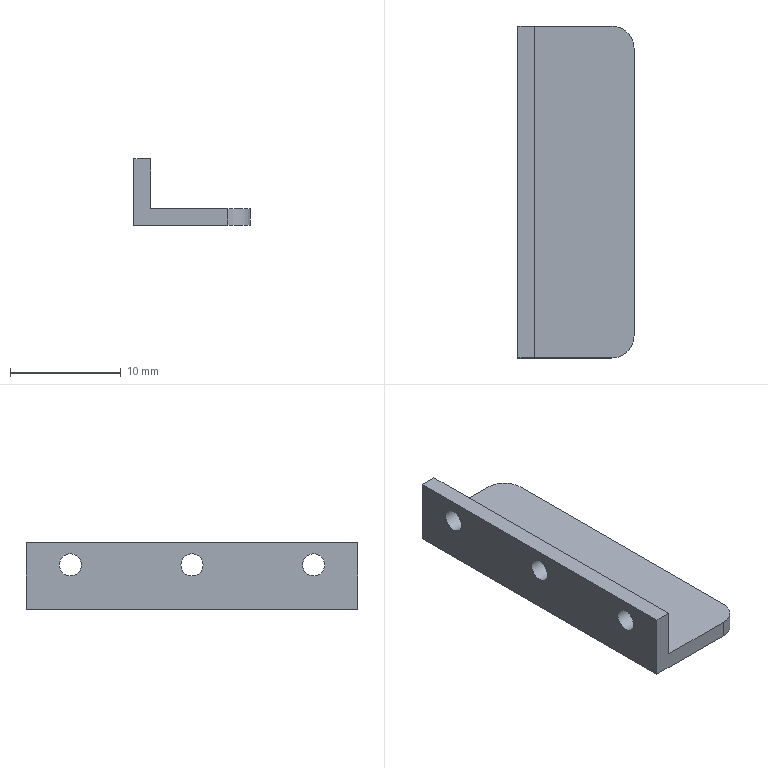Part | STEP file | 1-47.2 | 1 solid | 13 faces | box 10.5 x 30 x 6 mm | volume 658.288 mm3 | plane 8 | cylinder 5 | commonest cylinder face diameters 2 x3 4 x2
STEP:
#1=CARTESIAN_POINT('',(0.,0.,0.));
#2=DIRECTION('',(0.,0.,1.));
#3=DIRECTION('',(1.,0.,0.));
#4=AXIS2_PLACEMENT_3D('',#1,#2,#3);
#5=CARTESIAN_POINT('',(-1.5,-15.,-3.));
#6=VERTEX_POINT('',#5);
#7=CARTESIAN_POINT('',(-1.5,15.,-3.));
#8=VERTEX_POINT('',#7);
#9=CARTESIAN_POINT('',(-1.5,-15.,-3.));
#10=DIRECTION('',(0.,1.,0.));
#11=VECTOR('',#10,1.);
#12=LINE('',#9,#11);
#13=CARTESIAN_POINT('',(-1.5,0.,12.));
#14=DIRECTION('',(1.,0.,0.));
#15=DIRECTION('',(0.,1.,0.));
#16=AXIS2_PLACEMENT_3D('',#13,#14,#15);
#17=PLANE('',#16);
#18=CARTESIAN_POINT('',(-15.,-15.));
#19=DIRECTION('',(1.,0.));
#20=VECTOR('',#19,1.);
#21=LINE('',#18,#20);
#22=(GEOMETRIC_REPRESENTATION_CONTEXT(2)PARAMETRIC_REPRESENTATION_CONTEXT()REPRESENTATION_CONTEXT('',''));
#23=DEFINITIONAL_REPRESENTATION('',(#21),#22);
#24=PCURVE('',#17,#23);
#25=CARTESIAN_POINT('',(15.,0.,-3.));
#26=DIRECTION('',(0.,0.,1.));
#27=DIRECTION('',(0.,1.,0.));
#28=AXIS2_PLACEMENT_3D('',#25,#26,#27);
#29=PLANE('',#28);
#30=CARTESIAN_POINT('',(-15.,16.5));
#31=DIRECTION('',(1.,0.));
#32=VECTOR('',#31,1.);
#33=LINE('',#30,#32);
#34=(GEOMETRIC_REPRESENTATION_CONTEXT(2)PARAMETRIC_REPRESENTATION_CONTEXT()REPRESENTATION_CONTEXT('',''));
#35=DEFINITIONAL_REPRESENTATION('',(#33),#34);
#36=PCURVE('',#29,#35);
#37=SURFACE_CURVE('',#12,(#24,#36),.PCURVE_S1.);
#38=EDGE_CURVE('',#6,#8,#37,.T.);
#39=ORIENTED_EDGE('',*,*,#38,.T.);
#40=CARTESIAN_POINT('',(-1.5,15.,3.));
#41=VERTEX_POINT('',#40);
#42=CARTESIAN_POINT('',(-1.5,15.,-3.));
#43=DIRECTION('',(0.,0.,1.));
#44=VECTOR('',#43,1.);
#45=LINE('',#42,#44);
#46=CARTESIAN_POINT('',(15.,-15.));
#47=DIRECTION('',(0.,1.));
#48=VECTOR('',#47,1.);
#49=LINE('',#46,#48);
#50=(GEOMETRIC_REPRESENTATION_CONTEXT(2)PARAMETRIC_REPRESENTATION_CONTEXT()REPRESENTATION_CONTEXT('',''));
#51=DEFINITIONAL_REPRESENTATION('',(#49),#50);
#52=PCURVE('',#17,#51);
#53=CARTESIAN_POINT('',(3.75,15.,0.));
#54=DIRECTION('',(0.,-1.,0.));
#55=DIRECTION('',(0.,0.,1.));
#56=AXIS2_PLACEMENT_3D('',#53,#54,#55);
#57=PLANE('',#56);
#58=CARTESIAN_POINT('',(-3.,5.25));
#59=DIRECTION('',(1.,0.));
#60=VECTOR('',#59,1.);
#61=LINE('',#58,#60);
#62=(GEOMETRIC_REPRESENTATION_CONTEXT(2)PARAMETRIC_REPRESENTATION_CONTEXT()REPRESENTATION_CONTEXT('',''));
#63=DEFINITIONAL_REPRESENTATION('',(#61),#62);
#64=PCURVE('',#57,#63);
#65=SURFACE_CURVE('',#45,(#52,#64),.PCURVE_S1.);
#66=EDGE_CURVE('',#8,#41,#65,.T.);
#67=ORIENTED_EDGE('',*,*,#66,.T.);
#68=CARTESIAN_POINT('',(-1.5,-15.,3.));
#69=VERTEX_POINT('',#68);
#70=CARTESIAN_POINT('',(-1.5,15.,3.));
#71=DIRECTION('',(0.,-1.,0.));
#72=VECTOR('',#71,1.);
#73=LINE('',#70,#72);
#74=CARTESIAN_POINT('',(15.,-9.));
#75=DIRECTION('',(-1.,0.));
#76=VECTOR('',#75,1.);
#77=LINE('',#74,#76);
#78=(GEOMETRIC_REPRESENTATION_CONTEXT(2)PARAMETRIC_REPRESENTATION_CONTEXT()REPRESENTATION_CONTEXT('',''));
#79=DEFINITIONAL_REPRESENTATION('',(#77),#78);
#80=PCURVE('',#17,#79);
#81=CARTESIAN_POINT('',(-0.75,0.,3.));
#82=DIRECTION('',(0.,0.,-1.));
#83=DIRECTION('',(0.,-1.,0.));
#84=AXIS2_PLACEMENT_3D('',#81,#82,#83);
#85=PLANE('',#84);
#86=CARTESIAN_POINT('',(-15.,0.75));
#87=DIRECTION('',(1.,0.));
#88=VECTOR('',#87,1.);
#89=LINE('',#86,#88);
#90=(GEOMETRIC_REPRESENTATION_CONTEXT(2)PARAMETRIC_REPRESENTATION_CONTEXT()REPRESENTATION_CONTEXT('',''));
#91=DEFINITIONAL_REPRESENTATION('',(#89),#90);
#92=PCURVE('',#85,#91);
#93=SURFACE_CURVE('',#73,(#80,#92),.PCURVE_S1.);
#94=EDGE_CURVE('',#41,#69,#93,.T.);
#95=ORIENTED_EDGE('',*,*,#94,.T.);
#96=CARTESIAN_POINT('',(-1.5,-15.,3.));
#97=DIRECTION('',(0.,0.,-1.));
#98=VECTOR('',#97,1.);
#99=LINE('',#96,#98);
#100=CARTESIAN_POINT('',(-15.,-9.));
#101=DIRECTION('',(0.,-1.));
#102=VECTOR('',#101,1.);
#103=LINE('',#100,#102);
#104=(GEOMETRIC_REPRESENTATION_CONTEXT(2)PARAMETRIC_REPRESENTATION_CONTEXT()REPRESENTATION_CONTEXT('',''));
#105=DEFINITIONAL_REPRESENTATION('',(#103),#104);
#106=PCURVE('',#17,#105);
#107=CARTESIAN_POINT('',(3.75,-15.,0.));
#108=DIRECTION('',(0.,1.,0.));
#109=DIRECTION('',(0.,0.,-1.));
#110=AXIS2_PLACEMENT_3D('',#107,#108,#109);
#111=PLANE('',#110);
#112=CARTESIAN_POINT('',(-3.,5.25));
#113=DIRECTION('',(1.,0.));
#114=VECTOR('',#113,1.);
#115=LINE('',#112,#114);
#116=(GEOMETRIC_REPRESENTATION_CONTEXT(2)PARAMETRIC_REPRESENTATION_CONTEXT()REPRESENTATION_CONTEXT('',''));
#117=DEFINITIONAL_REPRESENTATION('',(#115),#116);
#118=PCURVE('',#111,#117);
#119=SURFACE_CURVE('',#99,(#106,#118),.PCURVE_S1.);
#120=EDGE_CURVE('',#69,#6,#119,.T.);
#121=ORIENTED_EDGE('',*,*,#120,.T.);
#122=EDGE_LOOP('',(#39,#67,#95,#121));
#123=FACE_BOUND('',#122,.F.);
#124=CARTESIAN_POINT('',(-1.5,1.,1.));
#125=VERTEX_POINT('',#124);
#126=CARTESIAN_POINT('',(-1.5,0.,1.));
#127=DIRECTION('',(-1.,0.,0.));
#128=DIRECTION('',(0.,1.,0.));
#129=AXIS2_PLACEMENT_3D('',#126,#127,#128);
#130=CIRCLE('',#129,1.);
#131=CARTESIAN_POINT('',(1.,-11.));
#132=CARTESIAN_POINT('',(1.,-12.732));
#133=CARTESIAN_POINT('',(-0.5,-11.866));
#134=CARTESIAN_POINT('',(-2.,-11.));
#135=CARTESIAN_POINT('',(-0.5,-10.134));
#136=CARTESIAN_POINT('',(1.,-9.268));
#137=CARTESIAN_POINT('',(1.,-11.));
#138=(BOUNDED_CURVE()B_SPLINE_CURVE(2,(#131,#132,#133,#134,#135,#136,#137),.UNSPECIFIED.,.T.,.F.)B_SPLINE_CURVE_WITH_KNOTS((1,2,2,2,2,1),(-2.094,0.,2.094,4.189,6.283,8.378),.UNSPECIFIED.)CURVE()GEOMETRIC_REPRESENTATION_ITEM()RATIONAL_B_SPLINE_CURVE((1.,0.5,1.,0.5,1.,0.5,1.))REPRESENTATION_ITEM(''));
#139=(GEOMETRIC_REPRESENTATION_CONTEXT(2)PARAMETRIC_REPRESENTATION_CONTEXT()REPRESENTATION_CONTEXT('',''));
#140=DEFINITIONAL_REPRESENTATION('',(#138),#139);
#141=PCURVE('',#17,#140);
#142=CARTESIAN_POINT('',(0.,0.,1.));
#143=DIRECTION('',(-1.,0.,0.));
#144=DIRECTION('',(0.,1.,0.));
#145=AXIS2_PLACEMENT_3D('',#142,#143,#144);
#146=CYLINDRICAL_SURFACE('',#145,1.);
#147=CARTESIAN_POINT('',(0.,1.5));
#148=DIRECTION('',(1.,0.));
#149=VECTOR('',#148,1.);
#150=LINE('',#147,#149);
#151=(GEOMETRIC_REPRESENTATION_CONTEXT(2)PARAMETRIC_REPRESENTATION_CONTEXT()REPRESENTATION_CONTEXT('',''));
#152=DEFINITIONAL_REPRESENTATION('',(#150),#151);
#153=PCURVE('',#146,#152);
#154=SURFACE_CURVE('',#130,(#141,#153),.PCURVE_S1.);
#155=EDGE_CURVE('',#125,#125,#154,.T.);
#156=ORIENTED_EDGE('',*,*,#155,.T.);
#157=EDGE_LOOP('',(#156));
#158=FACE_BOUND('',#157,.F.);
#159=CARTESIAN_POINT('',(-1.5,-10.,1.));
#160=VERTEX_POINT('',#159);
#161=CARTESIAN_POINT('',(-1.5,-11.,1.));
#162=DIRECTION('',(-1.,0.,0.));
#163=DIRECTION('',(0.,1.,0.));
#164=AXIS2_PLACEMENT_3D('',#161,#162,#163);
#165=CIRCLE('',#164,1.);
#166=CARTESIAN_POINT('',(-10.,-11.));
#167=CARTESIAN_POINT('',(-10.,-12.732));
#168=CARTESIAN_POINT('',(-11.5,-11.866));
#169=CARTESIAN_POINT('',(-13.,-11.));
#170=CARTESIAN_POINT('',(-11.5,-10.134));
#171=CARTESIAN_POINT('',(-10.,-9.268));
#172=CARTESIAN_POINT('',(-10.,-11.));
#173=(BOUNDED_CURVE()B_SPLINE_CURVE(2,(#166,#167,#168,#169,#170,#171,#172),.UNSPECIFIED.,.T.,.F.)B_SPLINE_CURVE_WITH_KNOTS((1,2,2,2,2,1),(-2.094,0.,2.094,4.189,6.283,8.378),.UNSPECIFIED.)CURVE()GEOMETRIC_REPRESENTATION_ITEM()RATIONAL_B_SPLINE_CURVE((1.,0.5,1.,0.5,1.,0.5,1.))REPRESENTATION_ITEM(''));
#174=(GEOMETRIC_REPRESENTATION_CONTEXT(2)PARAMETRIC_REPRESENTATION_CONTEXT()REPRESENTATION_CONTEXT('',''));
#175=DEFINITIONAL_REPRESENTATION('',(#173),#174);
#176=PCURVE('',#17,#175);
#177=CARTESIAN_POINT('',(0.,-11.,1.));
#178=DIRECTION('',(-1.,0.,0.));
#179=DIRECTION('',(0.,1.,0.));
#180=AXIS2_PLACEMENT_3D('',#177,#178,#179);
#181=CYLINDRICAL_SURFACE('',#180,1.);
#182=CARTESIAN_POINT('',(0.,1.5));
#183=DIRECTION('',(1.,0.));
#184=VECTOR('',#183,1.);
#185=LINE('',#182,#184);
#186=(GEOMETRIC_REPRESENTATION_CONTEXT(2)PARAMETRIC_REPRESENTATION_CONTEXT()REPRESENTATION_CONTEXT('',''));
#187=DEFINITIONAL_REPRESENTATION('',(#185),#186);
#188=PCURVE('',#181,#187);
#189=SURFACE_CURVE('',#165,(#176,#188),.PCURVE_S1.);
#190=EDGE_CURVE('',#160,#160,#189,.T.);
#191=ORIENTED_EDGE('',*,*,#190,.T.);
#192=EDGE_LOOP('',(#191));
#193=FACE_BOUND('',#192,.F.);
#194=CARTESIAN_POINT('',(-1.5,12.,1.));
#195=VERTEX_POINT('',#194);
#196=CARTESIAN_POINT('',(-1.5,11.,1.));
#197=DIRECTION('',(-1.,0.,0.));
#198=DIRECTION('',(0.,1.,0.));
#199=AXIS2_PLACEMENT_3D('',#196,#197,#198);
#200=CIRCLE('',#199,1.);
#201=CARTESIAN_POINT('',(12.,-11.));
#202=CARTESIAN_POINT('',(12.,-12.732));
#203=CARTESIAN_POINT('',(10.5,-11.866));
#204=CARTESIAN_POINT('',(9.,-11.));
#205=CARTESIAN_POINT('',(10.5,-10.134));
#206=CARTESIAN_POINT('',(12.,-9.268));
#207=CARTESIAN_POINT('',(12.,-11.));
#208=(BOUNDED_CURVE()B_SPLINE_CURVE(2,(#201,#202,#203,#204,#205,#206,#207),.UNSPECIFIED.,.T.,.F.)B_SPLINE_CURVE_WITH_KNOTS((1,2,2,2,2,1),(-2.094,0.,2.094,4.189,6.283,8.378),.UNSPECIFIED.)CURVE()GEOMETRIC_REPRESENTATION_ITEM()RATIONAL_B_SPLINE_CURVE((1.,0.5,1.,0.5,1.,0.5,1.))REPRESENTATION_ITEM(''));
#209=(GEOMETRIC_REPRESENTATION_CONTEXT(2)PARAMETRIC_REPRESENTATION_CONTEXT()REPRESENTATION_CONTEXT('',''));
#210=DEFINITIONAL_REPRESENTATION('',(#208),#209);
#211=PCURVE('',#17,#210);
#212=CARTESIAN_POINT('',(0.,11.,1.));
#213=DIRECTION('',(-1.,0.,0.));
#214=DIRECTION('',(0.,1.,0.));
#215=AXIS2_PLACEMENT_3D('',#212,#213,#214);
#216=CYLINDRICAL_SURFACE('',#215,1.);
#217=CARTESIAN_POINT('',(0.,1.5));
#218=DIRECTION('',(1.,0.));
#219=VECTOR('',#218,1.);
#220=LINE('',#217,#219);
#221=(GEOMETRIC_REPRESENTATION_CONTEXT(2)PARAMETRIC_REPRESENTATION_CONTEXT()REPRESENTATION_CONTEXT('',''));
#222=DEFINITIONAL_REPRESENTATION('',(#220),#221);
#223=PCURVE('',#216,#222);
#224=SURFACE_CURVE('',#200,(#211,#223),.PCURVE_S1.);
#225=EDGE_CURVE('',#195,#195,#224,.T.);
#226=ORIENTED_EDGE('',*,*,#225,.T.);
#227=EDGE_LOOP('',(#226));
#228=FACE_BOUND('',#227,.F.);
#229=ADVANCED_FACE('',(#123,#158,#193,#228),#17,.F.);
#230=CARTESIAN_POINT('',(0.,15.,3.));
#231=VERTEX_POINT('',#230);
#232=CARTESIAN_POINT('',(0.,-15.,3.));
#233=VERTEX_POINT('',#232);
#234=CARTESIAN_POINT('',(0.,15.,3.));
#235=DIRECTION('',(0.,-1.,0.));
#236=VECTOR('',#235,1.);
#237=LINE('',#234,#236);
#238=CARTESIAN_POINT('',(-15.,-0.75));
#239=DIRECTION('',(1.,0.));
#240=VECTOR('',#239,1.);
#241=LINE('',#238,#240);
#242=(GEOMETRIC_REPRESENTATION_CONTEXT(2)PARAMETRIC_REPRESENTATION_CONTEXT()REPRESENTATION_CONTEXT('',''));
#243=DEFINITIONAL_REPRESENTATION('',(#241),#242);
#244=PCURVE('',#85,#243);
#245=CARTESIAN_POINT('',(0.,0.,12.));
#246=DIRECTION('',(1.,0.,0.));
#247=DIRECTION('',(0.,1.,0.));
#248=AXIS2_PLACEMENT_3D('',#245,#246,#247);
#249=PLANE('',#248);
#250=CARTESIAN_POINT('',(15.,-9.));
#251=DIRECTION('',(-1.,0.));
#252=VECTOR('',#251,1.);
#253=LINE('',#250,#252);
#254=(GEOMETRIC_REPRESENTATION_CONTEXT(2)PARAMETRIC_REPRESENTATION_CONTEXT()REPRESENTATION_CONTEXT('',''));
#255=DEFINITIONAL_REPRESENTATION('',(#253),#254);
#256=PCURVE('',#249,#255);
#257=SURFACE_CURVE('',#237,(#244,#256),.PCURVE_S1.);
#258=EDGE_CURVE('',#231,#233,#257,.T.);
#259=ORIENTED_EDGE('',*,*,#258,.T.);
#260=CARTESIAN_POINT('',(0.,-15.,3.));
#261=DIRECTION('',(-1.,0.,0.));
#262=VECTOR('',#261,1.);
#263=LINE('',#260,#262);
#264=CARTESIAN_POINT('',(15.,-0.75));
#265=DIRECTION('',(0.,1.));
#266=VECTOR('',#265,1.);
#267=LINE('',#264,#266);
#268=(GEOMETRIC_REPRESENTATION_CONTEXT(2)PARAMETRIC_REPRESENTATION_CONTEXT()REPRESENTATION_CONTEXT('',''));
#269=DEFINITIONAL_REPRESENTATION('',(#267),#268);
#270=PCURVE('',#85,#269);
#271=CARTESIAN_POINT('',(-3.,3.75));
#272=DIRECTION('',(0.,1.));
#273=VECTOR('',#272,1.);
#274=LINE('',#271,#273);
#275=(GEOMETRIC_REPRESENTATION_CONTEXT(2)PARAMETRIC_REPRESENTATION_CONTEXT()REPRESENTATION_CONTEXT('',''));
#276=DEFINITIONAL_REPRESENTATION('',(#274),#275);
#277=PCURVE('',#111,#276);
#278=SURFACE_CURVE('',#263,(#270,#277),.PCURVE_S1.);
#279=EDGE_CURVE('',#233,#69,#278,.T.);
#280=ORIENTED_EDGE('',*,*,#279,.T.);
#281=ORIENTED_EDGE('',*,*,#94,.F.);
#282=CARTESIAN_POINT('',(0.,15.,3.));
#283=DIRECTION('',(-1.,0.,0.));
#284=VECTOR('',#283,1.);
#285=LINE('',#282,#284);
#286=CARTESIAN_POINT('',(-15.,-0.75));
#287=DIRECTION('',(0.,1.));
#288=VECTOR('',#287,1.);
#289=LINE('',#286,#288);
#290=(GEOMETRIC_REPRESENTATION_CONTEXT(2)PARAMETRIC_REPRESENTATION_CONTEXT()REPRESENTATION_CONTEXT('',''));
#291=DEFINITIONAL_REPRESENTATION('',(#289),#290);
#292=PCURVE('',#85,#291);
#293=CARTESIAN_POINT('',(3.,3.75));
#294=DIRECTION('',(0.,1.));
#295=VECTOR('',#294,1.);
#296=LINE('',#293,#295);
#297=(GEOMETRIC_REPRESENTATION_CONTEXT(2)PARAMETRIC_REPRESENTATION_CONTEXT()REPRESENTATION_CONTEXT('',''));
#298=DEFINITIONAL_REPRESENTATION('',(#296),#297);
#299=PCURVE('',#57,#298);
#300=SURFACE_CURVE('',#285,(#292,#299),.PCURVE_S1.);
#301=EDGE_CURVE('',#231,#41,#300,.T.);
#302=ORIENTED_EDGE('',*,*,#301,.F.);
#303=EDGE_LOOP('',(#259,#280,#281,#302));
#304=FACE_BOUND('',#303,.F.);
#305=ADVANCED_FACE('',(#304),#85,.F.);
#306=CARTESIAN_POINT('',(0.,1.,1.));
#307=VERTEX_POINT('',#306);
#308=CARTESIAN_POINT('',(0.,0.,1.));
#309=DIRECTION('',(-1.,0.,0.));
#310=DIRECTION('',(0.,1.,0.));
#311=AXIS2_PLACEMENT_3D('',#308,#309,#310);
#312=CIRCLE('',#311,1.);
#313=CARTESIAN_POINT('',(0.,0.));
#314=DIRECTION('',(1.,0.));
#315=VECTOR('',#314,1.);
#316=LINE('',#313,#315);
#317=(GEOMETRIC_REPRESENTATION_CONTEXT(2)PARAMETRIC_REPRESENTATION_CONTEXT()REPRESENTATION_CONTEXT('',''));
#318=DEFINITIONAL_REPRESENTATION('',(#316),#317);
#319=PCURVE('',#146,#318);
#320=CARTESIAN_POINT('',(1.,-11.));
#321=CARTESIAN_POINT('',(1.,-12.732));
#322=CARTESIAN_POINT('',(-0.5,-11.866));
#323=CARTESIAN_POINT('',(-2.,-11.));
#324=CARTESIAN_POINT('',(-0.5,-10.134));
#325=CARTESIAN_POINT('',(1.,-9.268));
#326=CARTESIAN_POINT('',(1.,-11.));
#327=(BOUNDED_CURVE()B_SPLINE_CURVE(2,(#320,#321,#322,#323,#324,#325,#326),.UNSPECIFIED.,.T.,.F.)B_SPLINE_CURVE_WITH_KNOTS((1,2,2,2,2,1),(-2.094,0.,2.094,4.189,6.283,8.378),.UNSPECIFIED.)CURVE()GEOMETRIC_REPRESENTATION_ITEM()RATIONAL_B_SPLINE_CURVE((1.,0.5,1.,0.5,1.,0.5,1.))REPRESENTATION_ITEM(''));
#328=(GEOMETRIC_REPRESENTATION_CONTEXT(2)PARAMETRIC_REPRESENTATION_CONTEXT()REPRESENTATION_CONTEXT('',''));
#329=DEFINITIONAL_REPRESENTATION('',(#327),#328);
#330=PCURVE('',#249,#329);
#331=SURFACE_CURVE('',#312,(#319,#330),.PCURVE_S1.);
#332=EDGE_CURVE('',#307,#307,#331,.T.);
#333=ORIENTED_EDGE('',*,*,#332,.T.);
#334=CARTESIAN_POINT('',(0.,1.,1.));
#335=DIRECTION('',(-1.,0.,0.));
#336=VECTOR('',#335,1.);
#337=LINE('',#334,#336);
#338=CARTESIAN_POINT('',(6.283,0.));
#339=DIRECTION('',(0.,1.));
#340=VECTOR('',#339,1.);
#341=LINE('',#338,#340);
#342=(GEOMETRIC_REPRESENTATION_CONTEXT(2)PARAMETRIC_REPRESENTATION_CONTEXT()REPRESENTATION_CONTEXT('',''));
#343=DEFINITIONAL_REPRESENTATION('',(#341),#342);
#344=PCURVE('',#146,#343);
#345=CARTESIAN_POINT('',(0.,0.));
#346=DIRECTION('',(0.,1.));
#347=VECTOR('',#346,1.);
#348=LINE('',#345,#347);
#349=(GEOMETRIC_REPRESENTATION_CONTEXT(2)PARAMETRIC_REPRESENTATION_CONTEXT()REPRESENTATION_CONTEXT('',''));
#350=DEFINITIONAL_REPRESENTATION('',(#348),#349);
#351=PCURVE('',#146,#350);
#352=SEAM_CURVE('',#337,(#344,#351),.PCURVE_S1.);
#353=EDGE_CURVE('',#307,#125,#352,.T.);
#354=ORIENTED_EDGE('',*,*,#353,.T.);
#355=ORIENTED_EDGE('',*,*,#155,.F.);
#356=ORIENTED_EDGE('',*,*,#353,.F.);
#357=EDGE_LOOP('',(#333,#354,#355,#356));
#358=FACE_BOUND('',#357,.F.);
#359=ADVANCED_FACE('',(#358),#146,.F.);
#360=CARTESIAN_POINT('',(0.,-10.,1.));
#361=VERTEX_POINT('',#360);
#362=CARTESIAN_POINT('',(0.,-11.,1.));
#363=DIRECTION('',(-1.,0.,0.));
#364=DIRECTION('',(0.,1.,0.));
#365=AXIS2_PLACEMENT_3D('',#362,#363,#364);
#366=CIRCLE('',#365,1.);
#367=CARTESIAN_POINT('',(0.,0.));
#368=DIRECTION('',(1.,0.));
#369=VECTOR('',#368,1.);
#370=LINE('',#367,#369);
#371=(GEOMETRIC_REPRESENTATION_CONTEXT(2)PARAMETRIC_REPRESENTATION_CONTEXT()REPRESENTATION_CONTEXT('',''));
#372=DEFINITIONAL_REPRESENTATION('',(#370),#371);
#373=PCURVE('',#181,#372);
#374=CARTESIAN_POINT('',(-10.,-11.));
#375=CARTESIAN_POINT('',(-10.,-12.732));
#376=CARTESIAN_POINT('',(-11.5,-11.866));
#377=CARTESIAN_POINT('',(-13.,-11.));
#378=CARTESIAN_POINT('',(-11.5,-10.134));
#379=CARTESIAN_POINT('',(-10.,-9.268));
#380=CARTESIAN_POINT('',(-10.,-11.));
#381=(BOUNDED_CURVE()B_SPLINE_CURVE(2,(#374,#375,#376,#377,#378,#379,#380),.UNSPECIFIED.,.T.,.F.)B_SPLINE_CURVE_WITH_KNOTS((1,2,2,2,2,1),(-2.094,0.,2.094,4.189,6.283,8.378),.UNSPECIFIED.)CURVE()GEOMETRIC_REPRESENTATION_ITEM()RATIONAL_B_SPLINE_CURVE((1.,0.5,1.,0.5,1.,0.5,1.))REPRESENTATION_ITEM(''));
#382=(GEOMETRIC_REPRESENTATION_CONTEXT(2)PARAMETRIC_REPRESENTATION_CONTEXT()REPRESENTATION_CONTEXT('',''));
#383=DEFINITIONAL_REPRESENTATION('',(#381),#382);
#384=PCURVE('',#249,#383);
#385=SURFACE_CURVE('',#366,(#373,#384),.PCURVE_S1.);
#386=EDGE_CURVE('',#361,#361,#385,.T.);
#387=ORIENTED_EDGE('',*,*,#386,.T.);
#388=CARTESIAN_POINT('',(0.,-10.,1.));
#389=DIRECTION('',(-1.,0.,0.));
#390=VECTOR('',#389,1.);
#391=LINE('',#388,#390);
#392=CARTESIAN_POINT('',(6.283,0.));
#393=DIRECTION('',(0.,1.));
#394=VECTOR('',#393,1.);
#395=LINE('',#392,#394);
#396=(GEOMETRIC_REPRESENTATION_CONTEXT(2)PARAMETRIC_REPRESENTATION_CONTEXT()REPRESENTATION_CONTEXT('',''));
#397=DEFINITIONAL_REPRESENTATION('',(#395),#396);
#398=PCURVE('',#181,#397);
#399=CARTESIAN_POINT('',(0.,0.));
#400=DIRECTION('',(0.,1.));
#401=VECTOR('',#400,1.);
#402=LINE('',#399,#401);
#403=(GEOMETRIC_REPRESENTATION_CONTEXT(2)PARAMETRIC_REPRESENTATION_CONTEXT()REPRESENTATION_CONTEXT('',''));
#404=DEFINITIONAL_REPRESENTATION('',(#402),#403);
#405=PCURVE('',#181,#404);
#406=SEAM_CURVE('',#391,(#398,#405),.PCURVE_S1.);
#407=EDGE_CURVE('',#361,#160,#406,.T.);
#408=ORIENTED_EDGE('',*,*,#407,.T.);
#409=ORIENTED_EDGE('',*,*,#190,.F.);
#410=ORIENTED_EDGE('',*,*,#407,.F.);
#411=EDGE_LOOP('',(#387,#408,#409,#410));
#412=FACE_BOUND('',#411,.F.);
#413=ADVANCED_FACE('',(#412),#181,.F.);
#414=CARTESIAN_POINT('',(0.,12.,1.));
#415=VERTEX_POINT('',#414);
#416=CARTESIAN_POINT('',(0.,11.,1.));
#417=DIRECTION('',(-1.,0.,0.));
#418=DIRECTION('',(0.,1.,0.));
#419=AXIS2_PLACEMENT_3D('',#416,#417,#418);
#420=CIRCLE('',#419,1.);
#421=CARTESIAN_POINT('',(0.,0.));
#422=DIRECTION('',(1.,0.));
#423=VECTOR('',#422,1.);
#424=LINE('',#421,#423);
#425=(GEOMETRIC_REPRESENTATION_CONTEXT(2)PARAMETRIC_REPRESENTATION_CONTEXT()REPRESENTATION_CONTEXT('',''));
#426=DEFINITIONAL_REPRESENTATION('',(#424),#425);
#427=PCURVE('',#216,#426);
#428=CARTESIAN_POINT('',(12.,-11.));
#429=CARTESIAN_POINT('',(12.,-12.732));
#430=CARTESIAN_POINT('',(10.5,-11.866));
#431=CARTESIAN_POINT('',(9.,-11.));
#432=CARTESIAN_POINT('',(10.5,-10.134));
#433=CARTESIAN_POINT('',(12.,-9.268));
#434=CARTESIAN_POINT('',(12.,-11.));
#435=(BOUNDED_CURVE()B_SPLINE_CURVE(2,(#428,#429,#430,#431,#432,#433,#434),.UNSPECIFIED.,.T.,.F.)B_SPLINE_CURVE_WITH_KNOTS((1,2,2,2,2,1),(-2.094,0.,2.094,4.189,6.283,8.378),.UNSPECIFIED.)CURVE()GEOMETRIC_REPRESENTATION_ITEM()RATIONAL_B_SPLINE_CURVE((1.,0.5,1.,0.5,1.,0.5,1.))REPRESENTATION_ITEM(''));
#436=(GEOMETRIC_REPRESENTATION_CONTEXT(2)PARAMETRIC_REPRESENTATION_CONTEXT()REPRESENTATION_CONTEXT('',''));
#437=DEFINITIONAL_REPRESENTATION('',(#435),#436);
#438=PCURVE('',#249,#437);
#439=SURFACE_CURVE('',#420,(#427,#438),.PCURVE_S1.);
#440=EDGE_CURVE('',#415,#415,#439,.T.);
#441=ORIENTED_EDGE('',*,*,#440,.T.);
#442=CARTESIAN_POINT('',(0.,12.,1.));
#443=DIRECTION('',(-1.,0.,0.));
#444=VECTOR('',#443,1.);
#445=LINE('',#442,#444);
#446=CARTESIAN_POINT('',(6.283,0.));
#447=DIRECTION('',(0.,1.));
#448=VECTOR('',#447,1.);
#449=LINE('',#446,#448);
#450=(GEOMETRIC_REPRESENTATION_CONTEXT(2)PARAMETRIC_REPRESENTATION_CONTEXT()REPRESENTATION_CONTEXT('',''));
#451=DEFINITIONAL_REPRESENTATION('',(#449),#450);
#452=PCURVE('',#216,#451);
#453=CARTESIAN_POINT('',(0.,0.));
#454=DIRECTION('',(0.,1.));
#455=VECTOR('',#454,1.);
#456=LINE('',#453,#455);
#457=(GEOMETRIC_REPRESENTATION_CONTEXT(2)PARAMETRIC_REPRESENTATION_CONTEXT()REPRESENTATION_CONTEXT('',''));
#458=DEFINITIONAL_REPRESENTATION('',(#456),#457);
#459=PCURVE('',#216,#458);
#460=SEAM_CURVE('',#445,(#452,#459),.PCURVE_S1.);
#461=EDGE_CURVE('',#415,#195,#460,.T.);
#462=ORIENTED_EDGE('',*,*,#461,.T.);
#463=ORIENTED_EDGE('',*,*,#225,.F.);
#464=ORIENTED_EDGE('',*,*,#461,.F.);
#465=EDGE_LOOP('',(#441,#462,#463,#464));
#466=FACE_BOUND('',#465,.F.);
#467=ADVANCED_FACE('',(#466),#216,.F.);
#468=ORIENTED_EDGE('',*,*,#258,.T.);
#469=CARTESIAN_POINT('',(0.,-15.,-1.5));
#470=VERTEX_POINT('',#469);
#471=CARTESIAN_POINT('',(0.,-15.,3.));
#472=DIRECTION('',(0.,0.,-1.));
#473=VECTOR('',#472,1.);
#474=LINE('',#471,#473);
#475=CARTESIAN_POINT('',(-15.,-9.));
#476=DIRECTION('',(0.,-1.));
#477=VECTOR('',#476,1.);
#478=LINE('',#475,#477);
#479=(GEOMETRIC_REPRESENTATION_CONTEXT(2)PARAMETRIC_REPRESENTATION_CONTEXT()REPRESENTATION_CONTEXT('',''));
#480=DEFINITIONAL_REPRESENTATION('',(#478),#479);
#481=PCURVE('',#249,#480);
#482=CARTESIAN_POINT('',(-3.,3.75));
#483=DIRECTION('',(1.,0.));
#484=VECTOR('',#483,1.);
#485=LINE('',#482,#484);
#486=(GEOMETRIC_REPRESENTATION_CONTEXT(2)PARAMETRIC_REPRESENTATION_CONTEXT()REPRESENTATION_CONTEXT('',''));
#487=DEFINITIONAL_REPRESENTATION('',(#485),#486);
#488=PCURVE('',#111,#487);
#489=SURFACE_CURVE('',#474,(#481,#488),.PCURVE_S1.);
#490=EDGE_CURVE('',#233,#470,#489,.T.);
#491=ORIENTED_EDGE('',*,*,#490,.T.);
#492=CARTESIAN_POINT('',(0.,15.,-1.5));
#493=VERTEX_POINT('',#492);
#494=CARTESIAN_POINT('',(0.,-15.,-1.5));
#495=DIRECTION('',(0.,1.,0.));
#496=VECTOR('',#495,1.);
#497=LINE('',#494,#496);
#498=CARTESIAN_POINT('',(-15.,-13.5));
#499=DIRECTION('',(1.,0.));
#500=VECTOR('',#499,1.);
#501=LINE('',#498,#500);
#502=(GEOMETRIC_REPRESENTATION_CONTEXT(2)PARAMETRIC_REPRESENTATION_CONTEXT()REPRESENTATION_CONTEXT('',''));
#503=DEFINITIONAL_REPRESENTATION('',(#501),#502);
#504=PCURVE('',#249,#503);
#505=CARTESIAN_POINT('',(15.,1.682,-1.5));
#506=DIRECTION('',(0.,0.,-1.));
#507=DIRECTION('',(0.,1.,0.));
#508=AXIS2_PLACEMENT_3D('',#505,#506,#507);
#509=PLANE('',#508);
#510=CARTESIAN_POINT('',(-16.682,-15.));
#511=DIRECTION('',(1.,0.));
#512=VECTOR('',#511,1.);
#513=LINE('',#510,#512);
#514=(GEOMETRIC_REPRESENTATION_CONTEXT(2)PARAMETRIC_REPRESENTATION_CONTEXT()REPRESENTATION_CONTEXT('',''));
#515=DEFINITIONAL_REPRESENTATION('',(#513),#514);
#516=PCURVE('',#509,#515);
#517=SURFACE_CURVE('',#497,(#504,#516),.PCURVE_S1.);
#518=EDGE_CURVE('',#470,#493,#517,.T.);
#519=ORIENTED_EDGE('',*,*,#518,.T.);
#520=CARTESIAN_POINT('',(0.,15.,-1.5));
#521=DIRECTION('',(0.,0.,1.));
#522=VECTOR('',#521,1.);
#523=LINE('',#520,#522);
#524=CARTESIAN_POINT('',(15.,-13.5));
#525=DIRECTION('',(0.,1.));
#526=VECTOR('',#525,1.);
#527=LINE('',#524,#526);
#528=(GEOMETRIC_REPRESENTATION_CONTEXT(2)PARAMETRIC_REPRESENTATION_CONTEXT()REPRESENTATION_CONTEXT('',''));
#529=DEFINITIONAL_REPRESENTATION('',(#527),#528);
#530=PCURVE('',#249,#529);
#531=CARTESIAN_POINT('',(-1.5,3.75));
#532=DIRECTION('',(1.,0.));
#533=VECTOR('',#532,1.);
#534=LINE('',#531,#533);
#535=(GEOMETRIC_REPRESENTATION_CONTEXT(2)PARAMETRIC_REPRESENTATION_CONTEXT()REPRESENTATION_CONTEXT('',''));
#536=DEFINITIONAL_REPRESENTATION('',(#534),#535);
#537=PCURVE('',#57,#536);
#538=SURFACE_CURVE('',#523,(#530,#537),.PCURVE_S1.);
#539=EDGE_CURVE('',#493,#231,#538,.T.);
#540=ORIENTED_EDGE('',*,*,#539,.T.);
#541=EDGE_LOOP('',(#468,#491,#519,#540));
#542=FACE_BOUND('',#541,.T.);
#543=ORIENTED_EDGE('',*,*,#332,.T.);
#544=EDGE_LOOP('',(#543));
#545=FACE_BOUND('',#544,.T.);
#546=ORIENTED_EDGE('',*,*,#386,.T.);
#547=EDGE_LOOP('',(#546));
#548=FACE_BOUND('',#547,.T.);
#549=ORIENTED_EDGE('',*,*,#440,.T.);
#550=EDGE_LOOP('',(#549));
#551=FACE_BOUND('',#550,.T.);
#552=ADVANCED_FACE('',(#542,#545,#548,#551),#249,.T.);
#553=ORIENTED_EDGE('',*,*,#38,.F.);
#554=CARTESIAN_POINT('',(7.,-15.,-3.));
#555=VERTEX_POINT('',#554);
#556=CARTESIAN_POINT('',(-1.5,-15.,-3.));
#557=DIRECTION('',(1.,0.,0.));
#558=VECTOR('',#557,1.);
#559=LINE('',#556,#558);
#560=CARTESIAN_POINT('',(-15.,16.5));
#561=DIRECTION('',(0.,-1.));
#562=VECTOR('',#561,1.);
#563=LINE('',#560,#562);
#564=(GEOMETRIC_REPRESENTATION_CONTEXT(2)PARAMETRIC_REPRESENTATION_CONTEXT()REPRESENTATION_CONTEXT('',''));
#565=DEFINITIONAL_REPRESENTATION('',(#563),#564);
#566=PCURVE('',#29,#565);
#567=CARTESIAN_POINT('',(3.,5.25));
#568=DIRECTION('',(0.,-1.));
#569=VECTOR('',#568,1.);
#570=LINE('',#567,#569);
#571=(GEOMETRIC_REPRESENTATION_CONTEXT(2)PARAMETRIC_REPRESENTATION_CONTEXT()REPRESENTATION_CONTEXT('',''));
#572=DEFINITIONAL_REPRESENTATION('',(#570),#571);
#573=PCURVE('',#111,#572);
#574=SURFACE_CURVE('',#559,(#566,#573),.PCURVE_S1.);
#575=EDGE_CURVE('',#6,#555,#574,.T.);
#576=ORIENTED_EDGE('',*,*,#575,.T.);
#577=CARTESIAN_POINT('',(9.,-13.,-3.));
#578=VERTEX_POINT('',#577);
#579=CARTESIAN_POINT('',(7.,-13.,-3.));
#580=DIRECTION('',(0.,0.,-1.));
#581=DIRECTION('',(1.,0.,0.));
#582=AXIS2_PLACEMENT_3D('',#579,#580,#581);
#583=CIRCLE('',#582,2.);
#584=CARTESIAN_POINT('',(-13.,6.));
#585=CARTESIAN_POINT('',(-16.464,6.));
#586=CARTESIAN_POINT('',(-14.732,9.));
#587=CARTESIAN_POINT('',(-13.,12.));
#588=CARTESIAN_POINT('',(-11.268,9.));
#589=CARTESIAN_POINT('',(-9.536,6.));
#590=CARTESIAN_POINT('',(-13.,6.));
#591=(BOUNDED_CURVE()B_SPLINE_CURVE(2,(#584,#585,#586,#587,#588,#589,#590),.UNSPECIFIED.,.T.,.F.)B_SPLINE_CURVE_WITH_KNOTS((1,2,2,2,2,1),(-2.094,0.,2.094,4.189,6.283,8.378),.UNSPECIFIED.)CURVE()GEOMETRIC_REPRESENTATION_ITEM()RATIONAL_B_SPLINE_CURVE((1.,0.5,1.,0.5,1.,0.5,1.))REPRESENTATION_ITEM(''));
#592=(GEOMETRIC_REPRESENTATION_CONTEXT(2)PARAMETRIC_REPRESENTATION_CONTEXT()REPRESENTATION_CONTEXT('',''));
#593=DEFINITIONAL_REPRESENTATION('',(#591),#592);
#594=PCURVE('',#29,#593);
#595=CARTESIAN_POINT('',(7.,-13.,-3.));
#596=DIRECTION('',(0.,0.,1.));
#597=DIRECTION('',(1.,0.,0.));
#598=AXIS2_PLACEMENT_3D('',#595,#596,#597);
#599=CYLINDRICAL_SURFACE('',#598,2.);
#600=CARTESIAN_POINT('',(6.283,0.));
#601=DIRECTION('',(-1.,0.));
#602=VECTOR('',#601,1.);
#603=LINE('',#600,#602);
#604=(GEOMETRIC_REPRESENTATION_CONTEXT(2)PARAMETRIC_REPRESENTATION_CONTEXT()REPRESENTATION_CONTEXT('',''));
#605=DEFINITIONAL_REPRESENTATION('',(#603),#604);
#606=PCURVE('',#599,#605);
#607=SURFACE_CURVE('',#583,(#594,#606),.PCURVE_S1.);
#608=EDGE_CURVE('',#578,#555,#607,.T.);
#609=ORIENTED_EDGE('',*,*,#608,.F.);
#610=CARTESIAN_POINT('',(9.,13.,-3.));
#611=VERTEX_POINT('',#610);
#612=CARTESIAN_POINT('',(9.,13.,-3.));
#613=DIRECTION('',(0.,-1.,0.));
#614=VECTOR('',#613,1.);
#615=LINE('',#612,#614);
#616=CARTESIAN_POINT('',(13.,6.));
#617=DIRECTION('',(-1.,0.));
#618=VECTOR('',#617,1.);
#619=LINE('',#616,#618);
#620=(GEOMETRIC_REPRESENTATION_CONTEXT(2)PARAMETRIC_REPRESENTATION_CONTEXT()REPRESENTATION_CONTEXT('',''));
#621=DEFINITIONAL_REPRESENTATION('',(#619),#620);
#622=PCURVE('',#29,#621);
#623=CARTESIAN_POINT('',(9.,0.,0.));
#624=DIRECTION('',(-1.,0.,0.));
#625=DIRECTION('',(0.,-1.,0.));
#626=AXIS2_PLACEMENT_3D('',#623,#624,#625);
#627=PLANE('',#626);
#628=CARTESIAN_POINT('',(-13.,-3.));
#629=DIRECTION('',(1.,0.));
#630=VECTOR('',#629,1.);
#631=LINE('',#628,#630);
#632=(GEOMETRIC_REPRESENTATION_CONTEXT(2)PARAMETRIC_REPRESENTATION_CONTEXT()REPRESENTATION_CONTEXT('',''));
#633=DEFINITIONAL_REPRESENTATION('',(#631),#632);
#634=PCURVE('',#627,#633);
#635=SURFACE_CURVE('',#615,(#622,#634),.PCURVE_S1.);
#636=EDGE_CURVE('',#611,#578,#635,.T.);
#637=ORIENTED_EDGE('',*,*,#636,.F.);
#638=CARTESIAN_POINT('',(7.,15.,-3.));
#639=VERTEX_POINT('',#638);
#640=CARTESIAN_POINT('',(7.,13.,-3.));
#641=DIRECTION('',(0.,0.,-1.));
#642=DIRECTION('',(0.,1.,0.));
#643=AXIS2_PLACEMENT_3D('',#640,#641,#642);
#644=CIRCLE('',#643,2.);
#645=CARTESIAN_POINT('',(15.,8.));
#646=CARTESIAN_POINT('',(15.,4.536));
#647=CARTESIAN_POINT('',(12.,6.268));
#648=CARTESIAN_POINT('',(9.,8.));
#649=CARTESIAN_POINT('',(12.,9.732));
#650=CARTESIAN_POINT('',(15.,11.464));
#651=CARTESIAN_POINT('',(15.,8.));
#652=(BOUNDED_CURVE()B_SPLINE_CURVE(2,(#645,#646,#647,#648,#649,#650,#651),.UNSPECIFIED.,.T.,.F.)B_SPLINE_CURVE_WITH_KNOTS((1,2,2,2,2,1),(-2.094,0.,2.094,4.189,6.283,8.378),.UNSPECIFIED.)CURVE()GEOMETRIC_REPRESENTATION_ITEM()RATIONAL_B_SPLINE_CURVE((1.,0.5,1.,0.5,1.,0.5,1.))REPRESENTATION_ITEM(''));
#653=(GEOMETRIC_REPRESENTATION_CONTEXT(2)PARAMETRIC_REPRESENTATION_CONTEXT()REPRESENTATION_CONTEXT('',''));
#654=DEFINITIONAL_REPRESENTATION('',(#652),#653);
#655=PCURVE('',#29,#654);
#656=CARTESIAN_POINT('',(7.,13.,-3.));
#657=DIRECTION('',(0.,0.,1.));
#658=DIRECTION('',(0.,1.,0.));
#659=AXIS2_PLACEMENT_3D('',#656,#657,#658);
#660=CYLINDRICAL_SURFACE('',#659,2.);
#661=CARTESIAN_POINT('',(6.283,0.));
#662=DIRECTION('',(-1.,0.));
#663=VECTOR('',#662,1.);
#664=LINE('',#661,#663);
#665=(GEOMETRIC_REPRESENTATION_CONTEXT(2)PARAMETRIC_REPRESENTATION_CONTEXT()REPRESENTATION_CONTEXT('',''));
#666=DEFINITIONAL_REPRESENTATION('',(#664),#665);
#667=PCURVE('',#660,#666);
#668=SURFACE_CURVE('',#644,(#655,#667),.PCURVE_S1.);
#669=EDGE_CURVE('',#639,#611,#668,.T.);
#670=ORIENTED_EDGE('',*,*,#669,.F.);
#671=CARTESIAN_POINT('',(7.,15.,-3.));
#672=DIRECTION('',(-1.,0.,0.));
#673=VECTOR('',#672,1.);
#674=LINE('',#671,#673);
#675=CARTESIAN_POINT('',(15.,8.));
#676=DIRECTION('',(0.,1.));
#677=VECTOR('',#676,1.);
#678=LINE('',#675,#677);
#679=(GEOMETRIC_REPRESENTATION_CONTEXT(2)PARAMETRIC_REPRESENTATION_CONTEXT()REPRESENTATION_CONTEXT('',''));
#680=DEFINITIONAL_REPRESENTATION('',(#678),#679);
#681=PCURVE('',#29,#680);
#682=CARTESIAN_POINT('',(-3.,-3.25));
#683=DIRECTION('',(0.,1.));
#684=VECTOR('',#683,1.);
#685=LINE('',#682,#684);
#686=(GEOMETRIC_REPRESENTATION_CONTEXT(2)PARAMETRIC_REPRESENTATION_CONTEXT()REPRESENTATION_CONTEXT('',''));
#687=DEFINITIONAL_REPRESENTATION('',(#685),#686);
#688=PCURVE('',#57,#687);
#689=SURFACE_CURVE('',#674,(#681,#688),.PCURVE_S1.);
#690=EDGE_CURVE('',#639,#8,#689,.T.);
#691=ORIENTED_EDGE('',*,*,#690,.T.);
#692=EDGE_LOOP('',(#553,#576,#609,#637,#670,#691));
#693=FACE_BOUND('',#692,.F.);
#694=ADVANCED_FACE('',(#693),#29,.F.);
#695=ORIENTED_EDGE('',*,*,#539,.T.);
#696=ORIENTED_EDGE('',*,*,#301,.T.);
#697=ORIENTED_EDGE('',*,*,#66,.F.);
#698=ORIENTED_EDGE('',*,*,#690,.F.);
#699=CARTESIAN_POINT('',(7.,15.,-1.5));
#700=VERTEX_POINT('',#699);
#701=CARTESIAN_POINT('',(7.,15.,-3.));
#702=DIRECTION('',(0.,0.,1.));
#703=VECTOR('',#702,1.);
#704=LINE('',#701,#703);
#705=CARTESIAN_POINT('',(-3.,-3.25));
#706=DIRECTION('',(1.,0.));
#707=VECTOR('',#706,1.);
#708=LINE('',#705,#707);
#709=(GEOMETRIC_REPRESENTATION_CONTEXT(2)PARAMETRIC_REPRESENTATION_CONTEXT()REPRESENTATION_CONTEXT('',''));
#710=DEFINITIONAL_REPRESENTATION('',(#708),#709);
#711=PCURVE('',#57,#710);
#712=CARTESIAN_POINT('',(6.283,0.));
#713=DIRECTION('',(0.,1.));
#714=VECTOR('',#713,1.);
#715=LINE('',#712,#714);
#716=(GEOMETRIC_REPRESENTATION_CONTEXT(2)PARAMETRIC_REPRESENTATION_CONTEXT()REPRESENTATION_CONTEXT('',''));
#717=DEFINITIONAL_REPRESENTATION('',(#715),#716);
#718=PCURVE('',#660,#717);
#719=SURFACE_CURVE('',#704,(#711,#718),.PCURVE_S1.);
#720=EDGE_CURVE('',#639,#700,#719,.T.);
#721=ORIENTED_EDGE('',*,*,#720,.T.);
#722=CARTESIAN_POINT('',(0.,15.,-1.5));
#723=DIRECTION('',(1.,0.,0.));
#724=VECTOR('',#723,1.);
#725=LINE('',#722,#724);
#726=CARTESIAN_POINT('',(-1.5,3.75));
#727=DIRECTION('',(0.,-1.));
#728=VECTOR('',#727,1.);
#729=LINE('',#726,#728);
#730=(GEOMETRIC_REPRESENTATION_CONTEXT(2)PARAMETRIC_REPRESENTATION_CONTEXT()REPRESENTATION_CONTEXT('',''));
#731=DEFINITIONAL_REPRESENTATION('',(#729),#730);
#732=PCURVE('',#57,#731);
#733=CARTESIAN_POINT('',(13.318,-15.));
#734=DIRECTION('',(0.,1.));
#735=VECTOR('',#734,1.);
#736=LINE('',#733,#735);
#737=(GEOMETRIC_REPRESENTATION_CONTEXT(2)PARAMETRIC_REPRESENTATION_CONTEXT()REPRESENTATION_CONTEXT('',''));
#738=DEFINITIONAL_REPRESENTATION('',(#736),#737);
#739=PCURVE('',#509,#738);
#740=SURFACE_CURVE('',#725,(#732,#739),.PCURVE_S1.);
#741=EDGE_CURVE('',#493,#700,#740,.T.);
#742=ORIENTED_EDGE('',*,*,#741,.F.);
#743=EDGE_LOOP('',(#695,#696,#697,#698,#721,#742));
#744=FACE_BOUND('',#743,.F.);
#745=ADVANCED_FACE('',(#744),#57,.F.);
#746=ORIENTED_EDGE('',*,*,#120,.F.);
#747=ORIENTED_EDGE('',*,*,#279,.F.);
#748=ORIENTED_EDGE('',*,*,#490,.T.);
#749=CARTESIAN_POINT('',(7.,-15.,-1.5));
#750=VERTEX_POINT('',#749);
#751=CARTESIAN_POINT('',(7.,-15.,-1.5));
#752=DIRECTION('',(-1.,0.,0.));
#753=VECTOR('',#752,1.);
#754=LINE('',#751,#753);
#755=CARTESIAN_POINT('',(1.5,-3.25));
#756=DIRECTION('',(0.,1.));
#757=VECTOR('',#756,1.);
#758=LINE('',#755,#757);
#759=(GEOMETRIC_REPRESENTATION_CONTEXT(2)PARAMETRIC_REPRESENTATION_CONTEXT()REPRESENTATION_CONTEXT('',''));
#760=DEFINITIONAL_REPRESENTATION('',(#758),#759);
#761=PCURVE('',#111,#760);
#762=CARTESIAN_POINT('',(-16.682,-8.));
#763=DIRECTION('',(0.,-1.));
#764=VECTOR('',#763,1.);
#765=LINE('',#762,#764);
#766=(GEOMETRIC_REPRESENTATION_CONTEXT(2)PARAMETRIC_REPRESENTATION_CONTEXT()REPRESENTATION_CONTEXT('',''));
#767=DEFINITIONAL_REPRESENTATION('',(#765),#766);
#768=PCURVE('',#509,#767);
#769=SURFACE_CURVE('',#754,(#761,#768),.PCURVE_S1.);
#770=EDGE_CURVE('',#750,#470,#769,.T.);
#771=ORIENTED_EDGE('',*,*,#770,.F.);
#772=CARTESIAN_POINT('',(7.,-15.,-3.));
#773=DIRECTION('',(0.,0.,1.));
#774=VECTOR('',#773,1.);
#775=LINE('',#772,#774);
#776=CARTESIAN_POINT('',(3.,-3.25));
#777=DIRECTION('',(-1.,0.));
#778=VECTOR('',#777,1.);
#779=LINE('',#776,#778);
#780=(GEOMETRIC_REPRESENTATION_CONTEXT(2)PARAMETRIC_REPRESENTATION_CONTEXT()REPRESENTATION_CONTEXT('',''));
#781=DEFINITIONAL_REPRESENTATION('',(#779),#780);
#782=PCURVE('',#111,#781);
#783=CARTESIAN_POINT('',(4.712,0.));
#784=DIRECTION('',(0.,1.));
#785=VECTOR('',#784,1.);
#786=LINE('',#783,#785);
#787=(GEOMETRIC_REPRESENTATION_CONTEXT(2)PARAMETRIC_REPRESENTATION_CONTEXT()REPRESENTATION_CONTEXT('',''));
#788=DEFINITIONAL_REPRESENTATION('',(#786),#787);
#789=PCURVE('',#599,#788);
#790=SURFACE_CURVE('',#775,(#782,#789),.PCURVE_S1.);
#791=EDGE_CURVE('',#555,#750,#790,.T.);
#792=ORIENTED_EDGE('',*,*,#791,.F.);
#793=ORIENTED_EDGE('',*,*,#575,.F.);
#794=EDGE_LOOP('',(#746,#747,#748,#771,#792,#793));
#795=FACE_BOUND('',#794,.F.);
#796=ADVANCED_FACE('',(#795),#111,.F.);
#797=ORIENTED_EDGE('',*,*,#636,.T.);
#798=CARTESIAN_POINT('',(9.,-13.,-1.5));
#799=VERTEX_POINT('',#798);
#800=CARTESIAN_POINT('',(9.,-13.,-3.));
#801=DIRECTION('',(0.,0.,1.));
#802=VECTOR('',#801,1.);
#803=LINE('',#800,#802);
#804=CARTESIAN_POINT('',(13.,-3.));
#805=DIRECTION('',(0.,1.));
#806=VECTOR('',#805,1.);
#807=LINE('',#804,#806);
#808=(GEOMETRIC_REPRESENTATION_CONTEXT(2)PARAMETRIC_REPRESENTATION_CONTEXT()REPRESENTATION_CONTEXT('',''));
#809=DEFINITIONAL_REPRESENTATION('',(#807),#808);
#810=PCURVE('',#627,#809);
#811=CARTESIAN_POINT('',(6.283,0.));
#812=DIRECTION('',(0.,1.));
#813=VECTOR('',#812,1.);
#814=LINE('',#811,#813);
#815=(GEOMETRIC_REPRESENTATION_CONTEXT(2)PARAMETRIC_REPRESENTATION_CONTEXT()REPRESENTATION_CONTEXT('',''));
#816=DEFINITIONAL_REPRESENTATION('',(#814),#815);
#817=PCURVE('',#599,#816);
#818=SURFACE_CURVE('',#803,(#810,#817),.PCURVE_S1.);
#819=EDGE_CURVE('',#578,#799,#818,.T.);
#820=ORIENTED_EDGE('',*,*,#819,.T.);
#821=CARTESIAN_POINT('',(9.,13.,-1.5));
#822=VERTEX_POINT('',#821);
#823=CARTESIAN_POINT('',(9.,13.,-1.5));
#824=DIRECTION('',(0.,-1.,0.));
#825=VECTOR('',#824,1.);
#826=LINE('',#823,#825);
#827=CARTESIAN_POINT('',(-13.,-1.5));
#828=DIRECTION('',(1.,0.));
#829=VECTOR('',#828,1.);
#830=LINE('',#827,#829);
#831=(GEOMETRIC_REPRESENTATION_CONTEXT(2)PARAMETRIC_REPRESENTATION_CONTEXT()REPRESENTATION_CONTEXT('',''));
#832=DEFINITIONAL_REPRESENTATION('',(#830),#831);
#833=PCURVE('',#627,#832);
#834=CARTESIAN_POINT('',(11.318,-6.));
#835=DIRECTION('',(-1.,0.));
#836=VECTOR('',#835,1.);
#837=LINE('',#834,#836);
#838=(GEOMETRIC_REPRESENTATION_CONTEXT(2)PARAMETRIC_REPRESENTATION_CONTEXT()REPRESENTATION_CONTEXT('',''));
#839=DEFINITIONAL_REPRESENTATION('',(#837),#838);
#840=PCURVE('',#509,#839);
#841=SURFACE_CURVE('',#826,(#833,#840),.PCURVE_S1.);
#842=EDGE_CURVE('',#822,#799,#841,.T.);
#843=ORIENTED_EDGE('',*,*,#842,.F.);
#844=CARTESIAN_POINT('',(9.,13.,-3.));
#845=DIRECTION('',(0.,0.,1.));
#846=VECTOR('',#845,1.);
#847=LINE('',#844,#846);
#848=CARTESIAN_POINT('',(-13.,-3.));
#849=DIRECTION('',(0.,1.));
#850=VECTOR('',#849,1.);
#851=LINE('',#848,#850);
#852=(GEOMETRIC_REPRESENTATION_CONTEXT(2)PARAMETRIC_REPRESENTATION_CONTEXT()REPRESENTATION_CONTEXT('',''));
#853=DEFINITIONAL_REPRESENTATION('',(#851),#852);
#854=PCURVE('',#627,#853);
#855=CARTESIAN_POINT('',(4.712,0.));
#856=DIRECTION('',(0.,1.));
#857=VECTOR('',#856,1.);
#858=LINE('',#855,#857);
#859=(GEOMETRIC_REPRESENTATION_CONTEXT(2)PARAMETRIC_REPRESENTATION_CONTEXT()REPRESENTATION_CONTEXT('',''));
#860=DEFINITIONAL_REPRESENTATION('',(#858),#859);
#861=PCURVE('',#660,#860);
#862=SURFACE_CURVE('',#847,(#854,#861),.PCURVE_S1.);
#863=EDGE_CURVE('',#611,#822,#862,.T.);
#864=ORIENTED_EDGE('',*,*,#863,.F.);
#865=EDGE_LOOP('',(#797,#820,#843,#864));
#866=FACE_BOUND('',#865,.F.);
#867=ADVANCED_FACE('',(#866),#627,.F.);
#868=ORIENTED_EDGE('',*,*,#518,.T.);
#869=ORIENTED_EDGE('',*,*,#741,.T.);
#870=CARTESIAN_POINT('',(7.,13.,-1.5));
#871=DIRECTION('',(0.,0.,1.));
#872=DIRECTION('',(1.,0.,0.));
#873=AXIS2_PLACEMENT_3D('',#870,#871,#872);
#874=CIRCLE('',#873,2.);
#875=CARTESIAN_POINT('',(11.318,-6.));
#876=CARTESIAN_POINT('',(14.782,-6.));
#877=CARTESIAN_POINT('',(13.05,-9.));
#878=CARTESIAN_POINT('',(11.318,-12.));
#879=CARTESIAN_POINT('',(9.586,-9.));
#880=CARTESIAN_POINT('',(7.854,-6.));
#881=CARTESIAN_POINT('',(11.318,-6.));
#882=(BOUNDED_CURVE()B_SPLINE_CURVE(2,(#875,#876,#877,#878,#879,#880,#881),.UNSPECIFIED.,.T.,.F.)B_SPLINE_CURVE_WITH_KNOTS((1,2,2,2,2,1),(-2.094,0.,2.094,4.189,6.283,8.378),.UNSPECIFIED.)CURVE()GEOMETRIC_REPRESENTATION_ITEM()RATIONAL_B_SPLINE_CURVE((1.,0.5,1.,0.5,1.,0.5,1.))REPRESENTATION_ITEM(''));
#883=(GEOMETRIC_REPRESENTATION_CONTEXT(2)PARAMETRIC_REPRESENTATION_CONTEXT()REPRESENTATION_CONTEXT('',''));
#884=DEFINITIONAL_REPRESENTATION('',(#882),#883);
#885=PCURVE('',#509,#884);
#886=CARTESIAN_POINT('',(4.712,1.5));
#887=DIRECTION('',(1.,0.));
#888=VECTOR('',#887,1.);
#889=LINE('',#886,#888);
#890=(GEOMETRIC_REPRESENTATION_CONTEXT(2)PARAMETRIC_REPRESENTATION_CONTEXT()REPRESENTATION_CONTEXT('',''));
#891=DEFINITIONAL_REPRESENTATION('',(#889),#890);
#892=PCURVE('',#660,#891);
#893=SURFACE_CURVE('',#874,(#885,#892),.PCURVE_S1.);
#894=EDGE_CURVE('',#822,#700,#893,.T.);
#895=ORIENTED_EDGE('',*,*,#894,.F.);
#896=ORIENTED_EDGE('',*,*,#842,.T.);
#897=CARTESIAN_POINT('',(7.,-13.,-1.5));
#898=DIRECTION('',(0.,0.,1.));
#899=DIRECTION('',(0.,-1.,0.));
#900=AXIS2_PLACEMENT_3D('',#897,#898,#899);
#901=CIRCLE('',#900,2.);
#902=CARTESIAN_POINT('',(-16.682,-8.));
#903=CARTESIAN_POINT('',(-16.682,-4.536));
#904=CARTESIAN_POINT('',(-13.682,-6.268));
#905=CARTESIAN_POINT('',(-10.682,-8.));
#906=CARTESIAN_POINT('',(-13.682,-9.732));
#907=CARTESIAN_POINT('',(-16.682,-11.464));
#908=CARTESIAN_POINT('',(-16.682,-8.));
#909=(BOUNDED_CURVE()B_SPLINE_CURVE(2,(#902,#903,#904,#905,#906,#907,#908),.UNSPECIFIED.,.T.,.F.)B_SPLINE_CURVE_WITH_KNOTS((1,2,2,2,2,1),(-2.094,0.,2.094,4.189,6.283,8.378),.UNSPECIFIED.)CURVE()GEOMETRIC_REPRESENTATION_ITEM()RATIONAL_B_SPLINE_CURVE((1.,0.5,1.,0.5,1.,0.5,1.))REPRESENTATION_ITEM(''));
#910=(GEOMETRIC_REPRESENTATION_CONTEXT(2)PARAMETRIC_REPRESENTATION_CONTEXT()REPRESENTATION_CONTEXT('',''));
#911=DEFINITIONAL_REPRESENTATION('',(#909),#910);
#912=PCURVE('',#509,#911);
#913=CARTESIAN_POINT('',(4.712,1.5));
#914=DIRECTION('',(1.,0.));
#915=VECTOR('',#914,1.);
#916=LINE('',#913,#915);
#917=(GEOMETRIC_REPRESENTATION_CONTEXT(2)PARAMETRIC_REPRESENTATION_CONTEXT()REPRESENTATION_CONTEXT('',''));
#918=DEFINITIONAL_REPRESENTATION('',(#916),#917);
#919=PCURVE('',#599,#918);
#920=SURFACE_CURVE('',#901,(#912,#919),.PCURVE_S1.);
#921=EDGE_CURVE('',#750,#799,#920,.T.);
#922=ORIENTED_EDGE('',*,*,#921,.F.);
#923=ORIENTED_EDGE('',*,*,#770,.T.);
#924=EDGE_LOOP('',(#868,#869,#895,#896,#922,#923));
#925=FACE_BOUND('',#924,.F.);
#926=ADVANCED_FACE('',(#925),#509,.F.);
#927=ORIENTED_EDGE('',*,*,#819,.T.);
#928=ORIENTED_EDGE('',*,*,#921,.F.);
#929=ORIENTED_EDGE('',*,*,#791,.F.);
#930=ORIENTED_EDGE('',*,*,#608,.F.);
#931=EDGE_LOOP('',(#927,#928,#929,#930));
#932=FACE_BOUND('',#931,.T.);
#933=ADVANCED_FACE('',(#932),#599,.T.);
#934=ORIENTED_EDGE('',*,*,#720,.T.);
#935=ORIENTED_EDGE('',*,*,#894,.F.);
#936=ORIENTED_EDGE('',*,*,#863,.F.);
#937=ORIENTED_EDGE('',*,*,#669,.F.);
#938=EDGE_LOOP('',(#934,#935,#936,#937));
#939=FACE_BOUND('',#938,.T.);
#940=ADVANCED_FACE('',(#939),#660,.T.);
#941=CLOSED_SHELL('',(#229,#305,#359,#413,#467,#552,#694,#745,#796,#867,#926,#933,#940));
#942=MANIFOLD_SOLID_BREP('',#941);
#943=(LENGTH_UNIT()NAMED_UNIT(*)SI_UNIT(.MILLI.,.METRE.));
#944=UNCERTAINTY_MEASURE_WITH_UNIT(LENGTH_MEASURE(0.0000001),#943,'','');
#945=(NAMED_UNIT(*)PLANE_ANGLE_UNIT()SI_UNIT($,.RADIAN.));
#946=(NAMED_UNIT(*)SI_UNIT($,.STERADIAN.)SOLID_ANGLE_UNIT());
#947=(GEOMETRIC_REPRESENTATION_CONTEXT(3)GLOBAL_UNCERTAINTY_ASSIGNED_CONTEXT((#944))GLOBAL_UNIT_ASSIGNED_CONTEXT((#943,#945,#946))REPRESENTATION_CONTEXT('',''));
#948=ADVANCED_BREP_SHAPE_REPRESENTATION('',(#4,#942),#947);